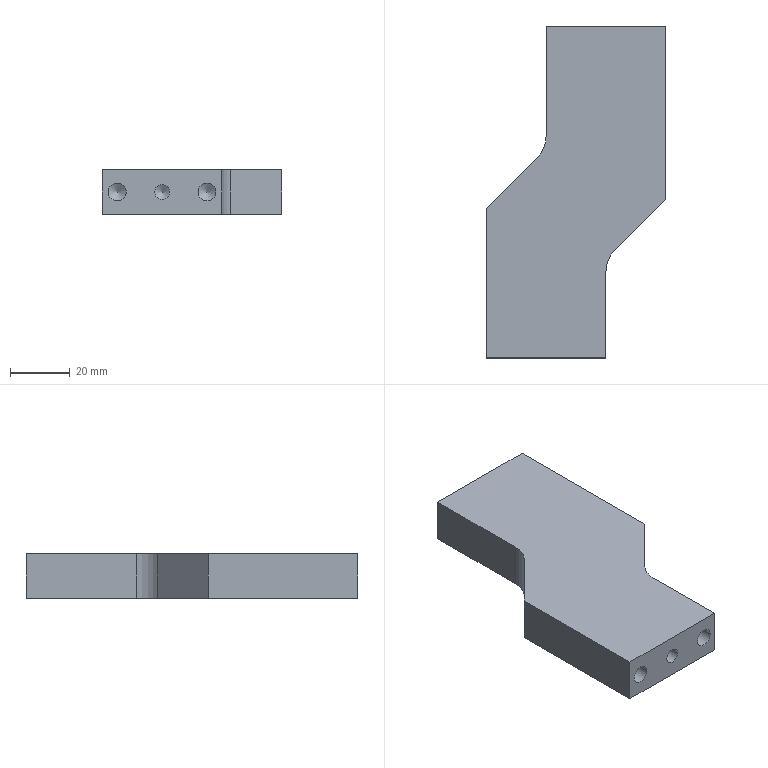Part | NX | features BREP 1 | 1 solid | 24 faces | box 60 x 111 x 15 mm | volume 69731 mm3 | plane 10 | cylinder 8 | cone 6 | commonest cylinder face diameters 6 x4 5 x2 20 x2
STEP:
#1=CARTESIAN_POINT('',(20.,0.,5.));
#2=VERTEX_POINT('',#1);
#3=CARTESIAN_POINT('',(20.,0.,7.5));
#4=DIRECTION('',(0.,-1.,0.));
#5=DIRECTION('',(0.,0.,-1.));
#6=AXIS2_PLACEMENT_3D('',#3,#4,#5);
#7=CIRCLE('',#6,2.5);
#8=EDGE_CURVE('',#2,#2,#7,.T.);
#9=ORIENTED_EDGE('',*,*,#8,.F.);
#10=EDGE_LOOP('',(#9));
#11=FACE_BOUND('',#10,.T.);
#12=CARTESIAN_POINT('',(5.,0.,4.5));
#13=VERTEX_POINT('',#12);
#14=CARTESIAN_POINT('',(5.,0.,7.5));
#15=DIRECTION('',(0.,-1.,0.));
#16=DIRECTION('',(0.,0.,-1.));
#17=AXIS2_PLACEMENT_3D('',#14,#15,#16);
#18=CIRCLE('',#17,3.);
#19=EDGE_CURVE('',#13,#13,#18,.T.);
#20=ORIENTED_EDGE('',*,*,#19,.F.);
#21=EDGE_LOOP('',(#20));
#22=FACE_BOUND('',#21,.T.);
#23=CARTESIAN_POINT('',(35.,0.,4.5));
#24=VERTEX_POINT('',#23);
#25=CARTESIAN_POINT('',(35.,0.,7.5));
#26=DIRECTION('',(0.,-1.,0.));
#27=DIRECTION('',(0.,0.,-1.));
#28=AXIS2_PLACEMENT_3D('',#25,#26,#27);
#29=CIRCLE('',#28,3.);
#30=EDGE_CURVE('',#24,#24,#29,.T.);
#31=ORIENTED_EDGE('',*,*,#30,.F.);
#32=EDGE_LOOP('',(#31));
#33=FACE_BOUND('',#32,.T.);
#34=CARTESIAN_POINT('',(0.,0.,0.));
#35=VERTEX_POINT('',#34);
#36=CARTESIAN_POINT('',(40.,0.,0.));
#37=VERTEX_POINT('',#36);
#38=CARTESIAN_POINT('',(40.,0.,0.));
#39=DIRECTION('',(1.,0.,0.));
#40=VECTOR('',#39,1000.);
#41=LINE('',#38,#40);
#42=EDGE_CURVE('',#35,#37,#41,.T.);
#43=ORIENTED_EDGE('',*,*,#42,.T.);
#44=CARTESIAN_POINT('',(40.,0.,15.));
#45=VERTEX_POINT('',#44);
#46=CARTESIAN_POINT('',(40.,0.,15.));
#47=DIRECTION('',(0.,0.,-1.));
#48=VECTOR('',#47,1000.);
#49=LINE('',#46,#48);
#50=EDGE_CURVE('',#45,#37,#49,.T.);
#51=ORIENTED_EDGE('',*,*,#50,.F.);
#52=CARTESIAN_POINT('',(0.,0.,15.));
#53=VERTEX_POINT('',#52);
#54=CARTESIAN_POINT('',(40.,0.,15.));
#55=DIRECTION('',(1.,0.,0.));
#56=VECTOR('',#55,1000.);
#57=LINE('',#54,#56);
#58=EDGE_CURVE('',#53,#45,#57,.T.);
#59=ORIENTED_EDGE('',*,*,#58,.F.);
#60=CARTESIAN_POINT('',(0.,0.,15.));
#61=DIRECTION('',(0.,0.,-1.));
#62=VECTOR('',#61,1000.);
#63=LINE('',#60,#62);
#64=EDGE_CURVE('',#53,#35,#63,.T.);
#65=ORIENTED_EDGE('',*,*,#64,.T.);
#66=EDGE_LOOP('',(#43,#51,#59,#65));
#67=FACE_BOUND('',#66,.T.);
#68=CARTESIAN_POINT('',(40.,0.,15.));
#69=DIRECTION('',(0.,1.,0.));
#70=DIRECTION('',(1.,0.,0.));
#71=AXIS2_PLACEMENT_3D('',#68,#69,#70);
#72=PLANE('',#71);
#73=ADVANCED_FACE('',(#11,#22,#33,#67),#72,.F.);
#74=CARTESIAN_POINT('',(40.,28.858,0.));
#75=VERTEX_POINT('',#74);
#76=CARTESIAN_POINT('',(40.,33.,0.));
#77=DIRECTION('',(0.,1.,0.));
#78=VECTOR('',#77,1000.);
#79=LINE('',#76,#78);
#80=EDGE_CURVE('',#37,#75,#79,.T.);
#81=ORIENTED_EDGE('',*,*,#80,.T.);
#82=CARTESIAN_POINT('',(40.,28.858,15.));
#83=VERTEX_POINT('',#82);
#84=CARTESIAN_POINT('',(40.,28.858,15.));
#85=DIRECTION('',(0.,0.,1.));
#86=VECTOR('',#85,1000.);
#87=LINE('',#84,#86);
#88=EDGE_CURVE('',#75,#83,#87,.T.);
#89=ORIENTED_EDGE('',*,*,#88,.T.);
#90=CARTESIAN_POINT('',(40.,33.,15.));
#91=DIRECTION('',(0.,1.,0.));
#92=VECTOR('',#91,1000.);
#93=LINE('',#90,#92);
#94=EDGE_CURVE('',#45,#83,#93,.T.);
#95=ORIENTED_EDGE('',*,*,#94,.F.);
#96=ORIENTED_EDGE('',*,*,#50,.T.);
#97=EDGE_LOOP('',(#81,#89,#95,#96));
#98=FACE_BOUND('',#97,.T.);
#99=CARTESIAN_POINT('',(40.,33.,15.));
#100=DIRECTION('',(-1.,0.,0.));
#101=DIRECTION('',(0.,1.,0.));
#102=AXIS2_PLACEMENT_3D('',#99,#100,#101);
#103=PLANE('',#102);
#104=ADVANCED_FACE('',(#98),#103,.F.);
#105=CARTESIAN_POINT('',(42.929,35.929,15.));
#106=VERTEX_POINT('',#105);
#107=CARTESIAN_POINT('',(60.,53.,15.));
#108=VERTEX_POINT('',#107);
#109=CARTESIAN_POINT('',(60.,53.,15.));
#110=DIRECTION('',(0.7071,0.7071,0.));
#111=VECTOR('',#110,1000.);
#112=LINE('',#109,#111);
#113=EDGE_CURVE('',#106,#108,#112,.T.);
#114=ORIENTED_EDGE('',*,*,#113,.F.);
#115=CARTESIAN_POINT('',(42.929,35.929,0.));
#116=VERTEX_POINT('',#115);
#117=CARTESIAN_POINT('',(42.929,35.929,0.));
#118=DIRECTION('',(0.,0.,-1.));
#119=VECTOR('',#118,1000.);
#120=LINE('',#117,#119);
#121=EDGE_CURVE('',#106,#116,#120,.T.);
#122=ORIENTED_EDGE('',*,*,#121,.T.);
#123=CARTESIAN_POINT('',(60.,53.,0.));
#124=VERTEX_POINT('',#123);
#125=CARTESIAN_POINT('',(60.,53.,0.));
#126=DIRECTION('',(0.7071,0.7071,0.));
#127=VECTOR('',#126,1000.);
#128=LINE('',#125,#127);
#129=EDGE_CURVE('',#116,#124,#128,.T.);
#130=ORIENTED_EDGE('',*,*,#129,.T.);
#131=CARTESIAN_POINT('',(60.,53.,15.));
#132=DIRECTION('',(0.,0.,-1.));
#133=VECTOR('',#132,1000.);
#134=LINE('',#131,#133);
#135=EDGE_CURVE('',#108,#124,#134,.T.);
#136=ORIENTED_EDGE('',*,*,#135,.F.);
#137=EDGE_LOOP('',(#114,#122,#130,#136));
#138=FACE_BOUND('',#137,.T.);
#139=CARTESIAN_POINT('',(60.,53.,15.));
#140=DIRECTION('',(-0.7071,0.7071,0.));
#141=DIRECTION('',(0.7071,0.7071,0.));
#142=AXIS2_PLACEMENT_3D('',#139,#140,#141);
#143=PLANE('',#142);
#144=ADVANCED_FACE('',(#138),#143,.F.);
#145=CARTESIAN_POINT('',(60.,111.,0.));
#146=VERTEX_POINT('',#145);
#147=CARTESIAN_POINT('',(60.,111.,0.));
#148=DIRECTION('',(0.,1.,0.));
#149=VECTOR('',#148,1000.);
#150=LINE('',#147,#149);
#151=EDGE_CURVE('',#124,#146,#150,.T.);
#152=ORIENTED_EDGE('',*,*,#151,.T.);
#153=CARTESIAN_POINT('',(60.,111.,15.));
#154=VERTEX_POINT('',#153);
#155=CARTESIAN_POINT('',(60.,111.,15.));
#156=DIRECTION('',(0.,0.,-1.));
#157=VECTOR('',#156,1000.);
#158=LINE('',#155,#157);
#159=EDGE_CURVE('',#154,#146,#158,.T.);
#160=ORIENTED_EDGE('',*,*,#159,.F.);
#161=CARTESIAN_POINT('',(60.,111.,15.));
#162=DIRECTION('',(0.,1.,0.));
#163=VECTOR('',#162,1000.);
#164=LINE('',#161,#163);
#165=EDGE_CURVE('',#108,#154,#164,.T.);
#166=ORIENTED_EDGE('',*,*,#165,.F.);
#167=ORIENTED_EDGE('',*,*,#135,.T.);
#168=EDGE_LOOP('',(#152,#160,#166,#167));
#169=FACE_BOUND('',#168,.T.);
#170=CARTESIAN_POINT('',(60.,111.,15.));
#171=DIRECTION('',(-1.,0.,0.));
#172=DIRECTION('',(0.,1.,0.));
#173=AXIS2_PLACEMENT_3D('',#170,#171,#172);
#174=PLANE('',#173);
#175=ADVANCED_FACE('',(#169),#174,.F.);
#176=CARTESIAN_POINT('',(40.,111.,10.));
#177=VERTEX_POINT('',#176);
#178=CARTESIAN_POINT('',(40.,111.,7.5));
#179=DIRECTION('',(0.,1.,0.));
#180=DIRECTION('',(0.,0.,1.));
#181=AXIS2_PLACEMENT_3D('',#178,#179,#180);
#182=CIRCLE('',#181,2.5);
#183=EDGE_CURVE('',#177,#177,#182,.T.);
#184=ORIENTED_EDGE('',*,*,#183,.F.);
#185=EDGE_LOOP('',(#184));
#186=FACE_BOUND('',#185,.T.);
#187=CARTESIAN_POINT('',(55.,111.,10.5));
#188=VERTEX_POINT('',#187);
#189=CARTESIAN_POINT('',(55.,111.,7.5));
#190=DIRECTION('',(0.,1.,0.));
#191=DIRECTION('',(0.,0.,1.));
#192=AXIS2_PLACEMENT_3D('',#189,#190,#191);
#193=CIRCLE('',#192,3.);
#194=EDGE_CURVE('',#188,#188,#193,.T.);
#195=ORIENTED_EDGE('',*,*,#194,.F.);
#196=EDGE_LOOP('',(#195));
#197=FACE_BOUND('',#196,.T.);
#198=CARTESIAN_POINT('',(25.,111.,10.5));
#199=VERTEX_POINT('',#198);
#200=CARTESIAN_POINT('',(25.,111.,7.5));
#201=DIRECTION('',(0.,1.,0.));
#202=DIRECTION('',(0.,0.,1.));
#203=AXIS2_PLACEMENT_3D('',#200,#201,#202);
#204=CIRCLE('',#203,3.);
#205=EDGE_CURVE('',#199,#199,#204,.T.);
#206=ORIENTED_EDGE('',*,*,#205,.F.);
#207=EDGE_LOOP('',(#206));
#208=FACE_BOUND('',#207,.T.);
#209=CARTESIAN_POINT('',(20.,111.,0.));
#210=VERTEX_POINT('',#209);
#211=CARTESIAN_POINT('',(20.,111.,0.));
#212=DIRECTION('',(-1.,0.,0.));
#213=VECTOR('',#212,1000.);
#214=LINE('',#211,#213);
#215=EDGE_CURVE('',#146,#210,#214,.T.);
#216=ORIENTED_EDGE('',*,*,#215,.T.);
#217=CARTESIAN_POINT('',(20.,111.,15.));
#218=VERTEX_POINT('',#217);
#219=CARTESIAN_POINT('',(20.,111.,15.));
#220=DIRECTION('',(0.,0.,-1.));
#221=VECTOR('',#220,1000.);
#222=LINE('',#219,#221);
#223=EDGE_CURVE('',#218,#210,#222,.T.);
#224=ORIENTED_EDGE('',*,*,#223,.F.);
#225=CARTESIAN_POINT('',(20.,111.,15.));
#226=DIRECTION('',(-1.,0.,0.));
#227=VECTOR('',#226,1000.);
#228=LINE('',#225,#227);
#229=EDGE_CURVE('',#154,#218,#228,.T.);
#230=ORIENTED_EDGE('',*,*,#229,.F.);
#231=ORIENTED_EDGE('',*,*,#159,.T.);
#232=EDGE_LOOP('',(#216,#224,#230,#231));
#233=FACE_BOUND('',#232,.T.);
#234=CARTESIAN_POINT('',(20.,111.,15.));
#235=DIRECTION('',(0.,-1.,0.));
#236=DIRECTION('',(0.,0.,1.));
#237=AXIS2_PLACEMENT_3D('',#234,#235,#236);
#238=PLANE('',#237);
#239=ADVANCED_FACE('',(#186,#197,#208,#233),#238,.F.);
#240=CARTESIAN_POINT('',(20.,74.142,0.));
#241=VERTEX_POINT('',#240);
#242=CARTESIAN_POINT('',(20.,70.,0.));
#243=DIRECTION('',(0.,-1.,0.));
#244=VECTOR('',#243,1000.);
#245=LINE('',#242,#244);
#246=EDGE_CURVE('',#210,#241,#245,.T.);
#247=ORIENTED_EDGE('',*,*,#246,.T.);
#248=CARTESIAN_POINT('',(20.,74.142,15.));
#249=VERTEX_POINT('',#248);
#250=CARTESIAN_POINT('',(20.,74.142,15.));
#251=DIRECTION('',(0.,0.,1.));
#252=VECTOR('',#251,1000.);
#253=LINE('',#250,#252);
#254=EDGE_CURVE('',#241,#249,#253,.T.);
#255=ORIENTED_EDGE('',*,*,#254,.T.);
#256=CARTESIAN_POINT('',(20.,70.,15.));
#257=DIRECTION('',(0.,-1.,0.));
#258=VECTOR('',#257,1000.);
#259=LINE('',#256,#258);
#260=EDGE_CURVE('',#218,#249,#259,.T.);
#261=ORIENTED_EDGE('',*,*,#260,.F.);
#262=ORIENTED_EDGE('',*,*,#223,.T.);
#263=EDGE_LOOP('',(#247,#255,#261,#262));
#264=FACE_BOUND('',#263,.T.);
#265=CARTESIAN_POINT('',(20.,70.,15.));
#266=DIRECTION('',(1.,0.,0.));
#267=DIRECTION('',(0.,0.,1.));
#268=AXIS2_PLACEMENT_3D('',#265,#266,#267);
#269=PLANE('',#268);
#270=ADVANCED_FACE('',(#264),#269,.F.);
#271=CARTESIAN_POINT('',(17.071,67.071,15.));
#272=VERTEX_POINT('',#271);
#273=CARTESIAN_POINT('',(0.,50.,15.));
#274=VERTEX_POINT('',#273);
#275=CARTESIAN_POINT('',(0.,50.,15.));
#276=DIRECTION('',(-0.7071,-0.7071,0.));
#277=VECTOR('',#276,1000.);
#278=LINE('',#275,#277);
#279=EDGE_CURVE('',#272,#274,#278,.T.);
#280=ORIENTED_EDGE('',*,*,#279,.F.);
#281=CARTESIAN_POINT('',(17.071,67.071,0.));
#282=VERTEX_POINT('',#281);
#283=CARTESIAN_POINT('',(17.071,67.071,0.));
#284=DIRECTION('',(0.,0.,-1.));
#285=VECTOR('',#284,1000.);
#286=LINE('',#283,#285);
#287=EDGE_CURVE('',#272,#282,#286,.T.);
#288=ORIENTED_EDGE('',*,*,#287,.T.);
#289=CARTESIAN_POINT('',(0.,50.,0.));
#290=VERTEX_POINT('',#289);
#291=CARTESIAN_POINT('',(0.,50.,0.));
#292=DIRECTION('',(-0.7071,-0.7071,0.));
#293=VECTOR('',#292,1000.);
#294=LINE('',#291,#293);
#295=EDGE_CURVE('',#282,#290,#294,.T.);
#296=ORIENTED_EDGE('',*,*,#295,.T.);
#297=CARTESIAN_POINT('',(0.,50.,15.));
#298=DIRECTION('',(0.,0.,-1.));
#299=VECTOR('',#298,1000.);
#300=LINE('',#297,#299);
#301=EDGE_CURVE('',#274,#290,#300,.T.);
#302=ORIENTED_EDGE('',*,*,#301,.F.);
#303=EDGE_LOOP('',(#280,#288,#296,#302));
#304=FACE_BOUND('',#303,.T.);
#305=CARTESIAN_POINT('',(0.,50.,15.));
#306=DIRECTION('',(0.7071,-0.7071,0.));
#307=DIRECTION('',(-0.7071,-0.7071,0.));
#308=AXIS2_PLACEMENT_3D('',#305,#306,#307);
#309=PLANE('',#308);
#310=ADVANCED_FACE('',(#304),#309,.F.);
#311=CARTESIAN_POINT('',(0.,0.,0.));
#312=DIRECTION('',(0.,-1.,0.));
#313=VECTOR('',#312,1000.);
#314=LINE('',#311,#313);
#315=EDGE_CURVE('',#290,#35,#314,.T.);
#316=ORIENTED_EDGE('',*,*,#315,.T.);
#317=ORIENTED_EDGE('',*,*,#64,.F.);
#318=CARTESIAN_POINT('',(0.,0.,15.));
#319=DIRECTION('',(0.,-1.,0.));
#320=VECTOR('',#319,1000.);
#321=LINE('',#318,#320);
#322=EDGE_CURVE('',#274,#53,#321,.T.);
#323=ORIENTED_EDGE('',*,*,#322,.F.);
#324=ORIENTED_EDGE('',*,*,#301,.T.);
#325=EDGE_LOOP('',(#316,#317,#323,#324));
#326=FACE_BOUND('',#325,.T.);
#327=CARTESIAN_POINT('',(0.,0.,15.));
#328=DIRECTION('',(1.,0.,0.));
#329=DIRECTION('',(0.,0.,1.));
#330=AXIS2_PLACEMENT_3D('',#327,#328,#329);
#331=PLANE('',#330);
#332=ADVANCED_FACE('',(#326),#331,.F.);
#333=ORIENTED_EDGE('',*,*,#58,.T.);
#334=ORIENTED_EDGE('',*,*,#94,.T.);
#335=CARTESIAN_POINT('',(50.,28.858,15.));
#336=DIRECTION('',(0.,0.,-1.));
#337=DIRECTION('',(-1.,0.,0.));
#338=AXIS2_PLACEMENT_3D('',#335,#336,#337);
#339=CIRCLE('',#338,10.);
#340=EDGE_CURVE('',#83,#106,#339,.T.);
#341=ORIENTED_EDGE('',*,*,#340,.T.);
#342=ORIENTED_EDGE('',*,*,#113,.T.);
#343=ORIENTED_EDGE('',*,*,#165,.T.);
#344=ORIENTED_EDGE('',*,*,#229,.T.);
#345=ORIENTED_EDGE('',*,*,#260,.T.);
#346=CARTESIAN_POINT('',(10.,74.142,15.));
#347=DIRECTION('',(0.,0.,-1.));
#348=DIRECTION('',(-1.,0.,0.));
#349=AXIS2_PLACEMENT_3D('',#346,#347,#348);
#350=CIRCLE('',#349,10.);
#351=EDGE_CURVE('',#249,#272,#350,.T.);
#352=ORIENTED_EDGE('',*,*,#351,.T.);
#353=ORIENTED_EDGE('',*,*,#279,.T.);
#354=ORIENTED_EDGE('',*,*,#322,.T.);
#355=EDGE_LOOP('',(#333,#334,#341,#342,#343,#344,#345,#352,#353,#354));
#356=FACE_BOUND('',#355,.T.);
#357=CARTESIAN_POINT('',(0.,0.,15.));
#358=DIRECTION('',(0.,0.,-1.));
#359=DIRECTION('',(1.,0.,0.));
#360=AXIS2_PLACEMENT_3D('',#357,#358,#359);
#361=PLANE('',#360);
#362=ADVANCED_FACE('',(#356),#361,.F.);
#363=ORIENTED_EDGE('',*,*,#42,.F.);
#364=ORIENTED_EDGE('',*,*,#315,.F.);
#365=ORIENTED_EDGE('',*,*,#295,.F.);
#366=CARTESIAN_POINT('',(10.,74.142,0.));
#367=DIRECTION('',(0.,0.,1.));
#368=DIRECTION('',(-1.,0.,0.));
#369=AXIS2_PLACEMENT_3D('',#366,#367,#368);
#370=CIRCLE('',#369,10.);
#371=EDGE_CURVE('',#282,#241,#370,.T.);
#372=ORIENTED_EDGE('',*,*,#371,.T.);
#373=ORIENTED_EDGE('',*,*,#246,.F.);
#374=ORIENTED_EDGE('',*,*,#215,.F.);
#375=ORIENTED_EDGE('',*,*,#151,.F.);
#376=ORIENTED_EDGE('',*,*,#129,.F.);
#377=CARTESIAN_POINT('',(50.,28.858,0.));
#378=DIRECTION('',(0.,0.,1.));
#379=DIRECTION('',(-1.,0.,0.));
#380=AXIS2_PLACEMENT_3D('',#377,#378,#379);
#381=CIRCLE('',#380,10.);
#382=EDGE_CURVE('',#116,#75,#381,.T.);
#383=ORIENTED_EDGE('',*,*,#382,.T.);
#384=ORIENTED_EDGE('',*,*,#80,.F.);
#385=EDGE_LOOP('',(#363,#364,#365,#372,#373,#374,#375,#376,#383,#384));
#386=FACE_BOUND('',#385,.T.);
#387=CARTESIAN_POINT('',(0.,0.,0.));
#388=DIRECTION('',(0.,0.,-1.));
#389=DIRECTION('',(1.,0.,0.));
#390=AXIS2_PLACEMENT_3D('',#387,#388,#389);
#391=PLANE('',#390);
#392=ADVANCED_FACE('',(#386),#391,.T.);
#393=ORIENTED_EDGE('',*,*,#340,.F.);
#394=ORIENTED_EDGE('',*,*,#88,.F.);
#395=ORIENTED_EDGE('',*,*,#382,.F.);
#396=ORIENTED_EDGE('',*,*,#121,.F.);
#397=EDGE_LOOP('',(#393,#394,#395,#396));
#398=FACE_BOUND('',#397,.T.);
#399=CARTESIAN_POINT('',(50.,28.858,15.));
#400=DIRECTION('',(0.,0.,1.));
#401=DIRECTION('',(-1.,0.,0.));
#402=AXIS2_PLACEMENT_3D('',#399,#400,#401);
#403=CYLINDRICAL_SURFACE('',#402,10.);
#404=ADVANCED_FACE('',(#398),#403,.F.);
#405=ORIENTED_EDGE('',*,*,#351,.F.);
#406=ORIENTED_EDGE('',*,*,#254,.F.);
#407=ORIENTED_EDGE('',*,*,#371,.F.);
#408=ORIENTED_EDGE('',*,*,#287,.F.);
#409=EDGE_LOOP('',(#405,#406,#407,#408));
#410=FACE_BOUND('',#409,.T.);
#411=CARTESIAN_POINT('',(10.,74.142,15.));
#412=DIRECTION('',(0.,0.,1.));
#413=DIRECTION('',(-1.,0.,0.));
#414=AXIS2_PLACEMENT_3D('',#411,#412,#413);
#415=CYLINDRICAL_SURFACE('',#414,10.);
#416=ADVANCED_FACE('',(#410),#415,.F.);
#417=CARTESIAN_POINT('',(25.,97.197,7.5));
#418=VERTEX_POINT('',#417);
#419=VERTEX_LOOP('',#418);
#420=FACE_BOUND('',#419,.T.);
#421=CARTESIAN_POINT('',(25.,99.,10.5));
#422=VERTEX_POINT('',#421);
#423=CARTESIAN_POINT('',(25.,99.,7.5));
#424=DIRECTION('',(0.,1.,0.));
#425=DIRECTION('',(0.,0.,1.));
#426=AXIS2_PLACEMENT_3D('',#423,#424,#425);
#427=CIRCLE('',#426,3.);
#428=EDGE_CURVE('',#422,#422,#427,.T.);
#429=ORIENTED_EDGE('',*,*,#428,.T.);
#430=EDGE_LOOP('',(#429));
#431=FACE_BOUND('',#430,.T.);
#432=CARTESIAN_POINT('',(25.,99.,7.5));
#433=DIRECTION('',(0.,1.,0.));
#434=DIRECTION('',(0.,0.,-1.));
#435=AXIS2_PLACEMENT_3D('',#432,#433,#434);
#436=CONICAL_SURFACE('',#435,3.,1.03);
#437=ADVANCED_FACE('',(#420,#431),#436,.F.);
#438=ORIENTED_EDGE('',*,*,#428,.F.);
#439=EDGE_LOOP('',(#438));
#440=FACE_BOUND('',#439,.T.);
#441=ORIENTED_EDGE('',*,*,#205,.T.);
#442=EDGE_LOOP('',(#441));
#443=FACE_BOUND('',#442,.T.);
#444=CARTESIAN_POINT('',(25.,111.,7.5));
#445=DIRECTION('',(0.,1.,0.));
#446=DIRECTION('',(0.,0.,-1.));
#447=AXIS2_PLACEMENT_3D('',#444,#445,#446);
#448=CYLINDRICAL_SURFACE('',#447,3.);
#449=ADVANCED_FACE('',(#440,#443),#448,.F.);
#450=CARTESIAN_POINT('',(55.,97.197,7.5));
#451=VERTEX_POINT('',#450);
#452=VERTEX_LOOP('',#451);
#453=FACE_BOUND('',#452,.T.);
#454=CARTESIAN_POINT('',(55.,99.,10.5));
#455=VERTEX_POINT('',#454);
#456=CARTESIAN_POINT('',(55.,99.,7.5));
#457=DIRECTION('',(0.,1.,0.));
#458=DIRECTION('',(0.,0.,1.));
#459=AXIS2_PLACEMENT_3D('',#456,#457,#458);
#460=CIRCLE('',#459,3.);
#461=EDGE_CURVE('',#455,#455,#460,.T.);
#462=ORIENTED_EDGE('',*,*,#461,.T.);
#463=EDGE_LOOP('',(#462));
#464=FACE_BOUND('',#463,.T.);
#465=CARTESIAN_POINT('',(55.,99.,7.5));
#466=DIRECTION('',(0.,1.,0.));
#467=DIRECTION('',(0.,0.,-1.));
#468=AXIS2_PLACEMENT_3D('',#465,#466,#467);
#469=CONICAL_SURFACE('',#468,3.,1.03);
#470=ADVANCED_FACE('',(#453,#464),#469,.F.);
#471=ORIENTED_EDGE('',*,*,#461,.F.);
#472=EDGE_LOOP('',(#471));
#473=FACE_BOUND('',#472,.T.);
#474=ORIENTED_EDGE('',*,*,#194,.T.);
#475=EDGE_LOOP('',(#474));
#476=FACE_BOUND('',#475,.T.);
#477=CARTESIAN_POINT('',(55.,111.,7.5));
#478=DIRECTION('',(0.,1.,0.));
#479=DIRECTION('',(0.,0.,-1.));
#480=AXIS2_PLACEMENT_3D('',#477,#478,#479);
#481=CYLINDRICAL_SURFACE('',#480,3.);
#482=ADVANCED_FACE('',(#473,#476),#481,.F.);
#483=CARTESIAN_POINT('',(40.,94.498,7.5));
#484=VERTEX_POINT('',#483);
#485=VERTEX_LOOP('',#484);
#486=FACE_BOUND('',#485,.T.);
#487=CARTESIAN_POINT('',(40.,96.,10.));
#488=VERTEX_POINT('',#487);
#489=CARTESIAN_POINT('',(40.,96.,7.5));
#490=DIRECTION('',(0.,1.,0.));
#491=DIRECTION('',(0.,0.,1.));
#492=AXIS2_PLACEMENT_3D('',#489,#490,#491);
#493=CIRCLE('',#492,2.5);
#494=EDGE_CURVE('',#488,#488,#493,.T.);
#495=ORIENTED_EDGE('',*,*,#494,.T.);
#496=EDGE_LOOP('',(#495));
#497=FACE_BOUND('',#496,.T.);
#498=CARTESIAN_POINT('',(40.,96.,7.5));
#499=DIRECTION('',(0.,1.,0.));
#500=DIRECTION('',(0.,0.,-1.));
#501=AXIS2_PLACEMENT_3D('',#498,#499,#500);
#502=CONICAL_SURFACE('',#501,2.5,1.03);
#503=ADVANCED_FACE('',(#486,#497),#502,.F.);
#504=ORIENTED_EDGE('',*,*,#494,.F.);
#505=EDGE_LOOP('',(#504));
#506=FACE_BOUND('',#505,.T.);
#507=ORIENTED_EDGE('',*,*,#183,.T.);
#508=EDGE_LOOP('',(#507));
#509=FACE_BOUND('',#508,.T.);
#510=CARTESIAN_POINT('',(40.,111.,7.5));
#511=DIRECTION('',(0.,1.,0.));
#512=DIRECTION('',(0.,0.,-1.));
#513=AXIS2_PLACEMENT_3D('',#510,#511,#512);
#514=CYLINDRICAL_SURFACE('',#513,2.5);
#515=ADVANCED_FACE('',(#506,#509),#514,.F.);
#516=CARTESIAN_POINT('',(35.,13.803,7.5));
#517=VERTEX_POINT('',#516);
#518=VERTEX_LOOP('',#517);
#519=FACE_BOUND('',#518,.T.);
#520=CARTESIAN_POINT('',(35.,12.,4.5));
#521=VERTEX_POINT('',#520);
#522=CARTESIAN_POINT('',(35.,12.,7.5));
#523=DIRECTION('',(0.,-1.,0.));
#524=DIRECTION('',(0.,0.,-1.));
#525=AXIS2_PLACEMENT_3D('',#522,#523,#524);
#526=CIRCLE('',#525,3.);
#527=EDGE_CURVE('',#521,#521,#526,.T.);
#528=ORIENTED_EDGE('',*,*,#527,.T.);
#529=EDGE_LOOP('',(#528));
#530=FACE_BOUND('',#529,.T.);
#531=CARTESIAN_POINT('',(35.,12.,7.5));
#532=DIRECTION('',(0.,-1.,0.));
#533=DIRECTION('',(0.,0.,1.));
#534=AXIS2_PLACEMENT_3D('',#531,#532,#533);
#535=CONICAL_SURFACE('',#534,3.,1.03);
#536=ADVANCED_FACE('',(#519,#530),#535,.F.);
#537=ORIENTED_EDGE('',*,*,#527,.F.);
#538=EDGE_LOOP('',(#537));
#539=FACE_BOUND('',#538,.T.);
#540=ORIENTED_EDGE('',*,*,#30,.T.);
#541=EDGE_LOOP('',(#540));
#542=FACE_BOUND('',#541,.T.);
#543=CARTESIAN_POINT('',(35.,0.,7.5));
#544=DIRECTION('',(0.,-1.,0.));
#545=DIRECTION('',(0.,0.,1.));
#546=AXIS2_PLACEMENT_3D('',#543,#544,#545);
#547=CYLINDRICAL_SURFACE('',#546,3.);
#548=ADVANCED_FACE('',(#539,#542),#547,.F.);
#549=CARTESIAN_POINT('',(5.,13.803,7.5));
#550=VERTEX_POINT('',#549);
#551=VERTEX_LOOP('',#550);
#552=FACE_BOUND('',#551,.T.);
#553=CARTESIAN_POINT('',(5.,12.,4.5));
#554=VERTEX_POINT('',#553);
#555=CARTESIAN_POINT('',(5.,12.,7.5));
#556=DIRECTION('',(0.,-1.,0.));
#557=DIRECTION('',(0.,0.,-1.));
#558=AXIS2_PLACEMENT_3D('',#555,#556,#557);
#559=CIRCLE('',#558,3.);
#560=EDGE_CURVE('',#554,#554,#559,.T.);
#561=ORIENTED_EDGE('',*,*,#560,.T.);
#562=EDGE_LOOP('',(#561));
#563=FACE_BOUND('',#562,.T.);
#564=CARTESIAN_POINT('',(5.,12.,7.5));
#565=DIRECTION('',(0.,-1.,0.));
#566=DIRECTION('',(0.,0.,1.));
#567=AXIS2_PLACEMENT_3D('',#564,#565,#566);
#568=CONICAL_SURFACE('',#567,3.,1.03);
#569=ADVANCED_FACE('',(#552,#563),#568,.F.);
#570=ORIENTED_EDGE('',*,*,#560,.F.);
#571=EDGE_LOOP('',(#570));
#572=FACE_BOUND('',#571,.T.);
#573=ORIENTED_EDGE('',*,*,#19,.T.);
#574=EDGE_LOOP('',(#573));
#575=FACE_BOUND('',#574,.T.);
#576=CARTESIAN_POINT('',(5.,0.,7.5));
#577=DIRECTION('',(0.,-1.,0.));
#578=DIRECTION('',(0.,0.,1.));
#579=AXIS2_PLACEMENT_3D('',#576,#577,#578);
#580=CYLINDRICAL_SURFACE('',#579,3.);
#581=ADVANCED_FACE('',(#572,#575),#580,.F.);
#582=CARTESIAN_POINT('',(20.,16.502,7.5));
#583=VERTEX_POINT('',#582);
#584=VERTEX_LOOP('',#583);
#585=FACE_BOUND('',#584,.T.);
#586=CARTESIAN_POINT('',(20.,15.,5.));
#587=VERTEX_POINT('',#586);
#588=CARTESIAN_POINT('',(20.,15.,7.5));
#589=DIRECTION('',(0.,-1.,0.));
#590=DIRECTION('',(0.,0.,-1.));
#591=AXIS2_PLACEMENT_3D('',#588,#589,#590);
#592=CIRCLE('',#591,2.5);
#593=EDGE_CURVE('',#587,#587,#592,.T.);
#594=ORIENTED_EDGE('',*,*,#593,.T.);
#595=EDGE_LOOP('',(#594));
#596=FACE_BOUND('',#595,.T.);
#597=CARTESIAN_POINT('',(20.,15.,7.5));
#598=DIRECTION('',(0.,-1.,0.));
#599=DIRECTION('',(0.,0.,1.));
#600=AXIS2_PLACEMENT_3D('',#597,#598,#599);
#601=CONICAL_SURFACE('',#600,2.5,1.03);
#602=ADVANCED_FACE('',(#585,#596),#601,.F.);
#603=ORIENTED_EDGE('',*,*,#593,.F.);
#604=EDGE_LOOP('',(#603));
#605=FACE_BOUND('',#604,.T.);
#606=ORIENTED_EDGE('',*,*,#8,.T.);
#607=EDGE_LOOP('',(#606));
#608=FACE_BOUND('',#607,.T.);
#609=CARTESIAN_POINT('',(20.,0.,7.5));
#610=DIRECTION('',(0.,-1.,0.));
#611=DIRECTION('',(0.,0.,1.));
#612=AXIS2_PLACEMENT_3D('',#609,#610,#611);
#613=CYLINDRICAL_SURFACE('',#612,2.5);
#614=ADVANCED_FACE('',(#605,#608),#613,.F.);
#615=CLOSED_SHELL('',(#73,#104,#144,#175,#239,#270,#310,#332,#362,#392,#404,#416,#437,#449,#470,#482,#503,#515,#536,#548,#569,#581,#602,#614));
#616=MANIFOLD_SOLID_BREP('',#615);
#617=(LENGTH_UNIT()NAMED_UNIT(*)SI_UNIT(.MILLI.,.METRE.));
#618=UNCERTAINTY_MEASURE_WITH_UNIT(LENGTH_MEASURE(0.00001),#617,'','');
#619=(NAMED_UNIT(*)PLANE_ANGLE_UNIT()SI_UNIT($,.RADIAN.));
#620=(NAMED_UNIT(*)SI_UNIT($,.STERADIAN.)SOLID_ANGLE_UNIT());
#621=(GEOMETRIC_REPRESENTATION_CONTEXT(3)GLOBAL_UNCERTAINTY_ASSIGNED_CONTEXT((#618))GLOBAL_UNIT_ASSIGNED_CONTEXT((#617,#619,#620))REPRESENTATION_CONTEXT('',''));
#622=ADVANCED_BREP_SHAPE_REPRESENTATION('',(#616),#621);